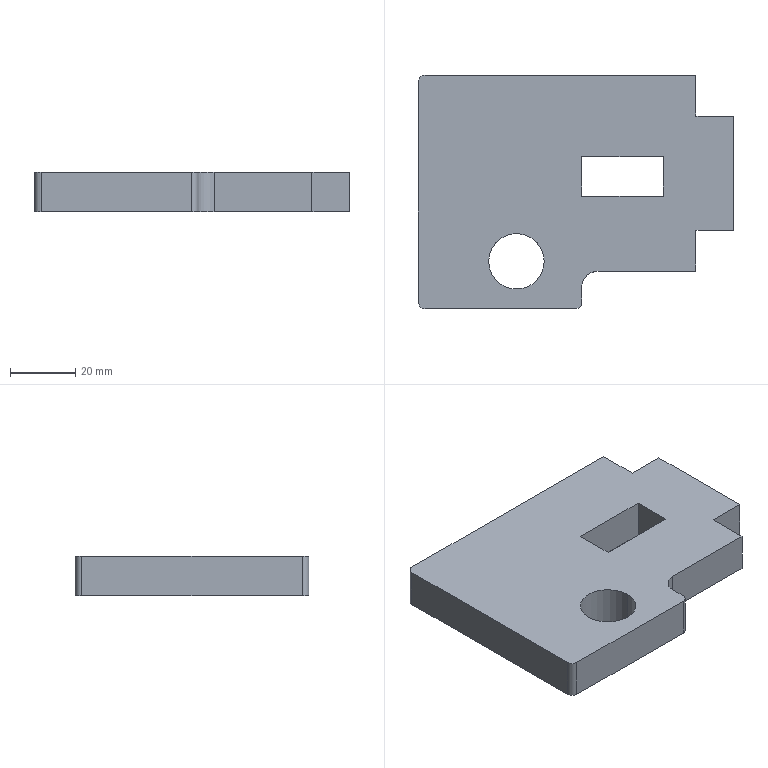Part | SolidWorks | features FlatPattern 1, SMBaseFlange 1, SheetMetal 1 | 1 solid | 22 faces | box 96.5 x 71.502 x 12 mm | volume 66641 mm3 | plane 16 | cylinder 6 | commonest cylinder face diameters 4 x3 17 x2 10 x1
STEP:
#1=CARTESIAN_POINT('',(-26.5,-18.,12.));
#2=VERTEX_POINT('',#1);
#3=CARTESIAN_POINT('',(-9.5,-18.,12.));
#4=VERTEX_POINT('',#3);
#5=CARTESIAN_POINT('',(-18.,-18.,12.));
#6=DIRECTION('',(0.,0.,1.));
#7=DIRECTION('',(1.,0.,0.));
#8=AXIS2_PLACEMENT_3D('',#5,#6,#7);
#9=CIRCLE('',#8,8.5);
#10=EDGE_CURVE('',#2,#4,#9,.T.);
#11=ORIENTED_EDGE('',*,*,#10,.T.);
#12=CARTESIAN_POINT('',(-9.5,-18.,0.));
#13=VERTEX_POINT('',#12);
#14=CARTESIAN_POINT('',(-9.5,-18.,12.));
#15=DIRECTION('',(0.,0.,-1.));
#16=VECTOR('',#15,1000.);
#17=LINE('',#14,#16);
#18=EDGE_CURVE('',#4,#13,#17,.T.);
#19=ORIENTED_EDGE('',*,*,#18,.T.);
#20=CARTESIAN_POINT('',(-26.5,-18.,0.));
#21=VERTEX_POINT('',#20);
#22=CARTESIAN_POINT('',(-18.,-18.,0.));
#23=DIRECTION('',(0.,0.,1.));
#24=DIRECTION('',(1.,0.,0.));
#25=AXIS2_PLACEMENT_3D('',#22,#23,#24);
#26=CIRCLE('',#25,8.5);
#27=EDGE_CURVE('',#21,#13,#26,.T.);
#28=ORIENTED_EDGE('',*,*,#27,.F.);
#29=CARTESIAN_POINT('',(-26.5,-18.,12.));
#30=DIRECTION('',(0.,0.,-1.));
#31=VECTOR('',#30,1000.);
#32=LINE('',#29,#31);
#33=EDGE_CURVE('',#2,#21,#32,.T.);
#34=ORIENTED_EDGE('',*,*,#33,.F.);
#35=EDGE_LOOP('',(#11,#19,#28,#34));
#36=FACE_OUTER_BOUND('',#35,.T.);
#37=CARTESIAN_POINT('',(-18.,-18.,12.));
#38=DIRECTION('',(0.,0.,-1.));
#39=DIRECTION('',(-1.,0.,0.));
#40=AXIS2_PLACEMENT_3D('',#37,#38,#39);
#41=CYLINDRICAL_SURFACE('',#40,8.5);
#42=ADVANCED_FACE('',(#36),#41,.F.);
#43=CARTESIAN_POINT('',(48.5,26.502,12.));
#44=VERTEX_POINT('',#43);
#45=CARTESIAN_POINT('',(37.,26.502,12.));
#46=VERTEX_POINT('',#45);
#47=CARTESIAN_POINT('',(48.5,26.502,12.));
#48=DIRECTION('',(-1.,0.,0.));
#49=VECTOR('',#48,1000.);
#50=LINE('',#47,#49);
#51=EDGE_CURVE('',#44,#46,#50,.T.);
#52=ORIENTED_EDGE('',*,*,#51,.T.);
#53=CARTESIAN_POINT('',(37.,39.002,12.));
#54=VERTEX_POINT('',#53);
#55=CARTESIAN_POINT('',(37.,26.502,12.));
#56=DIRECTION('',(0.,1.,0.));
#57=VECTOR('',#56,1000.);
#58=LINE('',#55,#57);
#59=EDGE_CURVE('',#46,#54,#58,.T.);
#60=ORIENTED_EDGE('',*,*,#59,.T.);
#61=CARTESIAN_POINT('',(-46.,39.002,12.));
#62=VERTEX_POINT('',#61);
#63=CARTESIAN_POINT('',(37.,39.002,12.));
#64=DIRECTION('',(-1.,0.,0.));
#65=VECTOR('',#64,1000.);
#66=LINE('',#63,#65);
#67=EDGE_CURVE('',#54,#62,#66,.T.);
#68=ORIENTED_EDGE('',*,*,#67,.T.);
#69=CARTESIAN_POINT('',(-48.,37.002,12.));
#70=VERTEX_POINT('',#69);
#71=CARTESIAN_POINT('',(-46.,37.002,12.));
#72=DIRECTION('',(0.,0.,1.));
#73=DIRECTION('',(1.,0.,0.));
#74=AXIS2_PLACEMENT_3D('',#71,#72,#73);
#75=CIRCLE('',#74,2.);
#76=EDGE_CURVE('',#62,#70,#75,.T.);
#77=ORIENTED_EDGE('',*,*,#76,.T.);
#78=CARTESIAN_POINT('',(-48.,-30.5,12.));
#79=VERTEX_POINT('',#78);
#80=CARTESIAN_POINT('',(-48.,-30.5,12.));
#81=DIRECTION('',(0.,-1.,0.));
#82=VECTOR('',#81,1000.);
#83=LINE('',#80,#82);
#84=EDGE_CURVE('',#70,#79,#83,.T.);
#85=ORIENTED_EDGE('',*,*,#84,.T.);
#86=CARTESIAN_POINT('',(-46.,-32.5,12.));
#87=VERTEX_POINT('',#86);
#88=CARTESIAN_POINT('',(-46.,-30.5,12.));
#89=DIRECTION('',(0.,0.,1.));
#90=DIRECTION('',(1.,0.,0.));
#91=AXIS2_PLACEMENT_3D('',#88,#89,#90);
#92=CIRCLE('',#91,2.);
#93=EDGE_CURVE('',#79,#87,#92,.T.);
#94=ORIENTED_EDGE('',*,*,#93,.T.);
#95=CARTESIAN_POINT('',(0.,-32.5,12.));
#96=VERTEX_POINT('',#95);
#97=CARTESIAN_POINT('',(-46.,-32.5,12.));
#98=DIRECTION('',(1.,0.,0.));
#99=VECTOR('',#98,1000.);
#100=LINE('',#97,#99);
#101=EDGE_CURVE('',#87,#96,#100,.T.);
#102=ORIENTED_EDGE('',*,*,#101,.T.);
#103=CARTESIAN_POINT('',(2.,-30.5,12.));
#104=VERTEX_POINT('',#103);
#105=CARTESIAN_POINT('',(0.,-30.5,12.));
#106=DIRECTION('',(0.,0.,1.));
#107=DIRECTION('',(1.,0.,0.));
#108=AXIS2_PLACEMENT_3D('',#105,#106,#107);
#109=CIRCLE('',#108,2.);
#110=EDGE_CURVE('',#96,#104,#109,.T.);
#111=ORIENTED_EDGE('',*,*,#110,.T.);
#112=CARTESIAN_POINT('',(2.,-25.998,12.));
#113=VERTEX_POINT('',#112);
#114=CARTESIAN_POINT('',(2.,-30.5,12.));
#115=DIRECTION('',(0.,1.,0.));
#116=VECTOR('',#115,1000.);
#117=LINE('',#114,#116);
#118=EDGE_CURVE('',#104,#113,#117,.T.);
#119=ORIENTED_EDGE('',*,*,#118,.T.);
#120=CARTESIAN_POINT('',(7.,-20.998,12.));
#121=VERTEX_POINT('',#120);
#122=CARTESIAN_POINT('',(7.,-25.998,12.));
#123=DIRECTION('',(0.,0.,-1.));
#124=DIRECTION('',(1.,0.,0.));
#125=AXIS2_PLACEMENT_3D('',#122,#123,#124);
#126=CIRCLE('',#125,5.);
#127=EDGE_CURVE('',#113,#121,#126,.T.);
#128=ORIENTED_EDGE('',*,*,#127,.T.);
#129=CARTESIAN_POINT('',(37.,-20.998,12.));
#130=VERTEX_POINT('',#129);
#131=CARTESIAN_POINT('',(7.,-20.998,12.));
#132=DIRECTION('',(1.,0.,0.));
#133=VECTOR('',#132,1000.);
#134=LINE('',#131,#133);
#135=EDGE_CURVE('',#121,#130,#134,.T.);
#136=ORIENTED_EDGE('',*,*,#135,.T.);
#137=CARTESIAN_POINT('',(37.,-8.498,12.));
#138=VERTEX_POINT('',#137);
#139=CARTESIAN_POINT('',(37.,-20.998,12.));
#140=DIRECTION('',(0.,1.,0.));
#141=VECTOR('',#140,1000.);
#142=LINE('',#139,#141);
#143=EDGE_CURVE('',#130,#138,#142,.T.);
#144=ORIENTED_EDGE('',*,*,#143,.T.);
#145=CARTESIAN_POINT('',(48.5,-8.498,12.));
#146=VERTEX_POINT('',#145);
#147=CARTESIAN_POINT('',(37.,-8.498,12.));
#148=DIRECTION('',(1.,0.,0.));
#149=VECTOR('',#148,1000.);
#150=LINE('',#147,#149);
#151=EDGE_CURVE('',#138,#146,#150,.T.);
#152=ORIENTED_EDGE('',*,*,#151,.T.);
#153=CARTESIAN_POINT('',(48.5,-8.498,12.));
#154=DIRECTION('',(0.,1.,0.));
#155=VECTOR('',#154,1000.);
#156=LINE('',#153,#155);
#157=EDGE_CURVE('',#146,#44,#156,.T.);
#158=ORIENTED_EDGE('',*,*,#157,.T.);
#159=EDGE_LOOP('',(#52,#60,#68,#77,#85,#94,#102,#111,#119,#128,#136,#144,#152,#158));
#160=FACE_OUTER_BOUND('',#159,.T.);
#161=ORIENTED_EDGE('',*,*,#10,.F.);
#162=CARTESIAN_POINT('',(-18.,-18.,12.));
#163=DIRECTION('',(0.,0.,1.));
#164=DIRECTION('',(1.,0.,0.));
#165=AXIS2_PLACEMENT_3D('',#162,#163,#164);
#166=CIRCLE('',#165,8.5);
#167=EDGE_CURVE('',#4,#2,#166,.T.);
#168=ORIENTED_EDGE('',*,*,#167,.F.);
#169=EDGE_LOOP('',(#161,#168));
#170=FACE_BOUND('',#169,.T.);
#171=CARTESIAN_POINT('',(2.,2.002,12.));
#172=VERTEX_POINT('',#171);
#173=CARTESIAN_POINT('',(27.,2.002,12.));
#174=VERTEX_POINT('',#173);
#175=CARTESIAN_POINT('',(2.,2.002,12.));
#176=DIRECTION('',(1.,0.,0.));
#177=VECTOR('',#176,1000.);
#178=LINE('',#175,#177);
#179=EDGE_CURVE('',#172,#174,#178,.T.);
#180=ORIENTED_EDGE('',*,*,#179,.F.);
#181=CARTESIAN_POINT('',(2.,14.002,12.));
#182=VERTEX_POINT('',#181);
#183=CARTESIAN_POINT('',(2.,14.002,12.));
#184=DIRECTION('',(0.,-1.,0.));
#185=VECTOR('',#184,1000.);
#186=LINE('',#183,#185);
#187=EDGE_CURVE('',#182,#172,#186,.T.);
#188=ORIENTED_EDGE('',*,*,#187,.F.);
#189=CARTESIAN_POINT('',(27.,14.002,12.));
#190=VERTEX_POINT('',#189);
#191=CARTESIAN_POINT('',(2.,14.002,12.));
#192=DIRECTION('',(-1.,0.,0.));
#193=VECTOR('',#192,1000.);
#194=LINE('',#191,#193);
#195=EDGE_CURVE('',#190,#182,#194,.T.);
#196=ORIENTED_EDGE('',*,*,#195,.F.);
#197=CARTESIAN_POINT('',(27.,14.002,12.));
#198=DIRECTION('',(0.,1.,0.));
#199=VECTOR('',#198,1000.);
#200=LINE('',#197,#199);
#201=EDGE_CURVE('',#174,#190,#200,.T.);
#202=ORIENTED_EDGE('',*,*,#201,.F.);
#203=EDGE_LOOP('',(#180,#188,#196,#202));
#204=FACE_BOUND('',#203,.T.);
#205=CARTESIAN_POINT('',(-46.,37.002,12.));
#206=DIRECTION('',(0.,0.,1.));
#207=DIRECTION('',(1.,0.,0.));
#208=AXIS2_PLACEMENT_3D('',#205,#206,#207);
#209=PLANE('',#208);
#210=ADVANCED_FACE('',(#160,#170,#204),#209,.T.);
#211=ORIENTED_EDGE('',*,*,#27,.T.);
#212=CARTESIAN_POINT('',(-18.,-18.,0.));
#213=DIRECTION('',(0.,0.,1.));
#214=DIRECTION('',(1.,0.,0.));
#215=AXIS2_PLACEMENT_3D('',#212,#213,#214);
#216=CIRCLE('',#215,8.5);
#217=EDGE_CURVE('',#13,#21,#216,.T.);
#218=ORIENTED_EDGE('',*,*,#217,.T.);
#219=EDGE_LOOP('',(#211,#218));
#220=FACE_BOUND('',#219,.T.);
#221=CARTESIAN_POINT('',(48.5,26.502,0.));
#222=VERTEX_POINT('',#221);
#223=CARTESIAN_POINT('',(37.,26.502,0.));
#224=VERTEX_POINT('',#223);
#225=CARTESIAN_POINT('',(48.5,26.502,0.));
#226=DIRECTION('',(-1.,0.,0.));
#227=VECTOR('',#226,1000.);
#228=LINE('',#225,#227);
#229=EDGE_CURVE('',#222,#224,#228,.T.);
#230=ORIENTED_EDGE('',*,*,#229,.F.);
#231=CARTESIAN_POINT('',(48.5,-8.498,0.));
#232=VERTEX_POINT('',#231);
#233=CARTESIAN_POINT('',(48.5,-8.498,0.));
#234=DIRECTION('',(0.,1.,0.));
#235=VECTOR('',#234,1000.);
#236=LINE('',#233,#235);
#237=EDGE_CURVE('',#232,#222,#236,.T.);
#238=ORIENTED_EDGE('',*,*,#237,.F.);
#239=CARTESIAN_POINT('',(37.,-8.498,0.));
#240=VERTEX_POINT('',#239);
#241=CARTESIAN_POINT('',(37.,-8.498,0.));
#242=DIRECTION('',(1.,0.,0.));
#243=VECTOR('',#242,1000.);
#244=LINE('',#241,#243);
#245=EDGE_CURVE('',#240,#232,#244,.T.);
#246=ORIENTED_EDGE('',*,*,#245,.F.);
#247=CARTESIAN_POINT('',(37.,-20.998,0.));
#248=VERTEX_POINT('',#247);
#249=CARTESIAN_POINT('',(37.,-20.998,0.));
#250=DIRECTION('',(0.,1.,0.));
#251=VECTOR('',#250,1000.);
#252=LINE('',#249,#251);
#253=EDGE_CURVE('',#248,#240,#252,.T.);
#254=ORIENTED_EDGE('',*,*,#253,.F.);
#255=CARTESIAN_POINT('',(7.,-20.998,0.));
#256=VERTEX_POINT('',#255);
#257=CARTESIAN_POINT('',(7.,-20.998,0.));
#258=DIRECTION('',(1.,0.,0.));
#259=VECTOR('',#258,1000.);
#260=LINE('',#257,#259);
#261=EDGE_CURVE('',#256,#248,#260,.T.);
#262=ORIENTED_EDGE('',*,*,#261,.F.);
#263=CARTESIAN_POINT('',(2.,-25.998,0.));
#264=VERTEX_POINT('',#263);
#265=CARTESIAN_POINT('',(7.,-25.998,0.));
#266=DIRECTION('',(0.,0.,-1.));
#267=DIRECTION('',(1.,0.,0.));
#268=AXIS2_PLACEMENT_3D('',#265,#266,#267);
#269=CIRCLE('',#268,5.);
#270=EDGE_CURVE('',#264,#256,#269,.T.);
#271=ORIENTED_EDGE('',*,*,#270,.F.);
#272=CARTESIAN_POINT('',(2.,-30.5,0.));
#273=VERTEX_POINT('',#272);
#274=CARTESIAN_POINT('',(2.,-30.5,0.));
#275=DIRECTION('',(0.,1.,0.));
#276=VECTOR('',#275,1000.);
#277=LINE('',#274,#276);
#278=EDGE_CURVE('',#273,#264,#277,.T.);
#279=ORIENTED_EDGE('',*,*,#278,.F.);
#280=CARTESIAN_POINT('',(0.,-32.5,0.));
#281=VERTEX_POINT('',#280);
#282=CARTESIAN_POINT('',(0.,-30.5,0.));
#283=DIRECTION('',(0.,0.,1.));
#284=DIRECTION('',(1.,0.,0.));
#285=AXIS2_PLACEMENT_3D('',#282,#283,#284);
#286=CIRCLE('',#285,2.);
#287=EDGE_CURVE('',#281,#273,#286,.T.);
#288=ORIENTED_EDGE('',*,*,#287,.F.);
#289=CARTESIAN_POINT('',(-46.,-32.5,0.));
#290=VERTEX_POINT('',#289);
#291=CARTESIAN_POINT('',(-46.,-32.5,0.));
#292=DIRECTION('',(1.,0.,0.));
#293=VECTOR('',#292,1000.);
#294=LINE('',#291,#293);
#295=EDGE_CURVE('',#290,#281,#294,.T.);
#296=ORIENTED_EDGE('',*,*,#295,.F.);
#297=CARTESIAN_POINT('',(-48.,-30.5,0.));
#298=VERTEX_POINT('',#297);
#299=CARTESIAN_POINT('',(-46.,-30.5,0.));
#300=DIRECTION('',(0.,0.,1.));
#301=DIRECTION('',(1.,0.,0.));
#302=AXIS2_PLACEMENT_3D('',#299,#300,#301);
#303=CIRCLE('',#302,2.);
#304=EDGE_CURVE('',#298,#290,#303,.T.);
#305=ORIENTED_EDGE('',*,*,#304,.F.);
#306=CARTESIAN_POINT('',(-48.,37.002,0.));
#307=VERTEX_POINT('',#306);
#308=CARTESIAN_POINT('',(-48.,-30.5,0.));
#309=DIRECTION('',(0.,-1.,0.));
#310=VECTOR('',#309,1000.);
#311=LINE('',#308,#310);
#312=EDGE_CURVE('',#307,#298,#311,.T.);
#313=ORIENTED_EDGE('',*,*,#312,.F.);
#314=CARTESIAN_POINT('',(-46.,39.002,0.));
#315=VERTEX_POINT('',#314);
#316=CARTESIAN_POINT('',(-46.,37.002,0.));
#317=DIRECTION('',(0.,0.,1.));
#318=DIRECTION('',(1.,0.,0.));
#319=AXIS2_PLACEMENT_3D('',#316,#317,#318);
#320=CIRCLE('',#319,2.);
#321=EDGE_CURVE('',#315,#307,#320,.T.);
#322=ORIENTED_EDGE('',*,*,#321,.F.);
#323=CARTESIAN_POINT('',(37.,39.002,0.));
#324=VERTEX_POINT('',#323);
#325=CARTESIAN_POINT('',(37.,39.002,0.));
#326=DIRECTION('',(-1.,0.,0.));
#327=VECTOR('',#326,1000.);
#328=LINE('',#325,#327);
#329=EDGE_CURVE('',#324,#315,#328,.T.);
#330=ORIENTED_EDGE('',*,*,#329,.F.);
#331=CARTESIAN_POINT('',(37.,26.502,0.));
#332=DIRECTION('',(0.,1.,0.));
#333=VECTOR('',#332,1000.);
#334=LINE('',#331,#333);
#335=EDGE_CURVE('',#224,#324,#334,.T.);
#336=ORIENTED_EDGE('',*,*,#335,.F.);
#337=EDGE_LOOP('',(#230,#238,#246,#254,#262,#271,#279,#288,#296,#305,#313,#322,#330,#336));
#338=FACE_OUTER_BOUND('',#337,.T.);
#339=CARTESIAN_POINT('',(2.,14.002,0.));
#340=VERTEX_POINT('',#339);
#341=CARTESIAN_POINT('',(2.,2.002,0.));
#342=VERTEX_POINT('',#341);
#343=CARTESIAN_POINT('',(2.,14.002,0.));
#344=DIRECTION('',(0.,-1.,0.));
#345=VECTOR('',#344,1000.);
#346=LINE('',#343,#345);
#347=EDGE_CURVE('',#340,#342,#346,.T.);
#348=ORIENTED_EDGE('',*,*,#347,.T.);
#349=CARTESIAN_POINT('',(27.,2.002,0.));
#350=VERTEX_POINT('',#349);
#351=CARTESIAN_POINT('',(2.,2.002,0.));
#352=DIRECTION('',(1.,0.,0.));
#353=VECTOR('',#352,1000.);
#354=LINE('',#351,#353);
#355=EDGE_CURVE('',#342,#350,#354,.T.);
#356=ORIENTED_EDGE('',*,*,#355,.T.);
#357=CARTESIAN_POINT('',(27.,14.002,0.));
#358=VERTEX_POINT('',#357);
#359=CARTESIAN_POINT('',(27.,14.002,0.));
#360=DIRECTION('',(0.,1.,0.));
#361=VECTOR('',#360,1000.);
#362=LINE('',#359,#361);
#363=EDGE_CURVE('',#350,#358,#362,.T.);
#364=ORIENTED_EDGE('',*,*,#363,.T.);
#365=CARTESIAN_POINT('',(2.,14.002,0.));
#366=DIRECTION('',(-1.,0.,0.));
#367=VECTOR('',#366,1000.);
#368=LINE('',#365,#367);
#369=EDGE_CURVE('',#358,#340,#368,.T.);
#370=ORIENTED_EDGE('',*,*,#369,.T.);
#371=EDGE_LOOP('',(#348,#356,#364,#370));
#372=FACE_BOUND('',#371,.T.);
#373=CARTESIAN_POINT('',(-46.,37.002,0.));
#374=DIRECTION('',(0.,0.,1.));
#375=DIRECTION('',(1.,0.,0.));
#376=AXIS2_PLACEMENT_3D('',#373,#374,#375);
#377=PLANE('',#376);
#378=ADVANCED_FACE('',(#220,#338,#372),#377,.F.);
#379=ORIENTED_EDGE('',*,*,#229,.T.);
#380=CARTESIAN_POINT('',(37.,26.502,12.));
#381=DIRECTION('',(0.,0.,-1.));
#382=VECTOR('',#381,1000.);
#383=LINE('',#380,#382);
#384=EDGE_CURVE('',#46,#224,#383,.T.);
#385=ORIENTED_EDGE('',*,*,#384,.F.);
#386=ORIENTED_EDGE('',*,*,#51,.F.);
#387=CARTESIAN_POINT('',(48.5,26.502,12.));
#388=DIRECTION('',(0.,0.,-1.));
#389=VECTOR('',#388,1000.);
#390=LINE('',#387,#389);
#391=EDGE_CURVE('',#44,#222,#390,.T.);
#392=ORIENTED_EDGE('',*,*,#391,.T.);
#393=EDGE_LOOP('',(#379,#385,#386,#392));
#394=FACE_OUTER_BOUND('',#393,.T.);
#395=CARTESIAN_POINT('',(48.5,26.502,12.));
#396=DIRECTION('',(0.,-1.,0.));
#397=DIRECTION('',(0.,0.,-1.));
#398=AXIS2_PLACEMENT_3D('',#395,#396,#397);
#399=PLANE('',#398);
#400=ADVANCED_FACE('',(#394),#399,.F.);
#401=ORIENTED_EDGE('',*,*,#335,.T.);
#402=CARTESIAN_POINT('',(37.,39.002,12.));
#403=DIRECTION('',(0.,0.,-1.));
#404=VECTOR('',#403,1000.);
#405=LINE('',#402,#404);
#406=EDGE_CURVE('',#54,#324,#405,.T.);
#407=ORIENTED_EDGE('',*,*,#406,.F.);
#408=ORIENTED_EDGE('',*,*,#59,.F.);
#409=ORIENTED_EDGE('',*,*,#384,.T.);
#410=EDGE_LOOP('',(#401,#407,#408,#409));
#411=FACE_OUTER_BOUND('',#410,.T.);
#412=CARTESIAN_POINT('',(37.,26.502,12.));
#413=DIRECTION('',(-1.,0.,0.));
#414=DIRECTION('',(0.,0.,1.));
#415=AXIS2_PLACEMENT_3D('',#412,#413,#414);
#416=PLANE('',#415);
#417=ADVANCED_FACE('',(#411),#416,.F.);
#418=ORIENTED_EDGE('',*,*,#329,.T.);
#419=CARTESIAN_POINT('',(-46.,39.002,12.));
#420=DIRECTION('',(0.,0.,-1.));
#421=VECTOR('',#420,1000.);
#422=LINE('',#419,#421);
#423=EDGE_CURVE('',#62,#315,#422,.T.);
#424=ORIENTED_EDGE('',*,*,#423,.F.);
#425=ORIENTED_EDGE('',*,*,#67,.F.);
#426=ORIENTED_EDGE('',*,*,#406,.T.);
#427=EDGE_LOOP('',(#418,#424,#425,#426));
#428=FACE_OUTER_BOUND('',#427,.T.);
#429=CARTESIAN_POINT('',(37.,39.002,12.));
#430=DIRECTION('',(0.,-1.,0.));
#431=DIRECTION('',(0.,0.,-1.));
#432=AXIS2_PLACEMENT_3D('',#429,#430,#431);
#433=PLANE('',#432);
#434=ADVANCED_FACE('',(#428),#433,.F.);
#435=ORIENTED_EDGE('',*,*,#321,.T.);
#436=CARTESIAN_POINT('',(-48.,37.002,12.));
#437=DIRECTION('',(0.,0.,-1.));
#438=VECTOR('',#437,1000.);
#439=LINE('',#436,#438);
#440=EDGE_CURVE('',#70,#307,#439,.T.);
#441=ORIENTED_EDGE('',*,*,#440,.F.);
#442=ORIENTED_EDGE('',*,*,#76,.F.);
#443=ORIENTED_EDGE('',*,*,#423,.T.);
#444=EDGE_LOOP('',(#435,#441,#442,#443));
#445=FACE_OUTER_BOUND('',#444,.T.);
#446=CARTESIAN_POINT('',(-46.,37.002,12.));
#447=DIRECTION('',(0.,0.,-1.));
#448=DIRECTION('',(-1.,0.,0.));
#449=AXIS2_PLACEMENT_3D('',#446,#447,#448);
#450=CYLINDRICAL_SURFACE('',#449,2.);
#451=ADVANCED_FACE('',(#445),#450,.T.);
#452=ORIENTED_EDGE('',*,*,#312,.T.);
#453=CARTESIAN_POINT('',(-48.,-30.5,12.));
#454=DIRECTION('',(0.,0.,-1.));
#455=VECTOR('',#454,1000.);
#456=LINE('',#453,#455);
#457=EDGE_CURVE('',#79,#298,#456,.T.);
#458=ORIENTED_EDGE('',*,*,#457,.F.);
#459=ORIENTED_EDGE('',*,*,#84,.F.);
#460=ORIENTED_EDGE('',*,*,#440,.T.);
#461=EDGE_LOOP('',(#452,#458,#459,#460));
#462=FACE_OUTER_BOUND('',#461,.T.);
#463=CARTESIAN_POINT('',(-48.,-30.5,12.));
#464=DIRECTION('',(1.,0.,0.));
#465=DIRECTION('',(0.,0.,-1.));
#466=AXIS2_PLACEMENT_3D('',#463,#464,#465);
#467=PLANE('',#466);
#468=ADVANCED_FACE('',(#462),#467,.F.);
#469=ORIENTED_EDGE('',*,*,#304,.T.);
#470=CARTESIAN_POINT('',(-46.,-32.5,12.));
#471=DIRECTION('',(0.,0.,-1.));
#472=VECTOR('',#471,1000.);
#473=LINE('',#470,#472);
#474=EDGE_CURVE('',#87,#290,#473,.T.);
#475=ORIENTED_EDGE('',*,*,#474,.F.);
#476=ORIENTED_EDGE('',*,*,#93,.F.);
#477=ORIENTED_EDGE('',*,*,#457,.T.);
#478=EDGE_LOOP('',(#469,#475,#476,#477));
#479=FACE_OUTER_BOUND('',#478,.T.);
#480=CARTESIAN_POINT('',(-46.,-30.5,12.));
#481=DIRECTION('',(0.,0.,-1.));
#482=DIRECTION('',(-1.,0.,0.));
#483=AXIS2_PLACEMENT_3D('',#480,#481,#482);
#484=CYLINDRICAL_SURFACE('',#483,2.);
#485=ADVANCED_FACE('',(#479),#484,.T.);
#486=ORIENTED_EDGE('',*,*,#295,.T.);
#487=CARTESIAN_POINT('',(0.,-32.5,12.));
#488=DIRECTION('',(0.,0.,-1.));
#489=VECTOR('',#488,1000.);
#490=LINE('',#487,#489);
#491=EDGE_CURVE('',#96,#281,#490,.T.);
#492=ORIENTED_EDGE('',*,*,#491,.F.);
#493=ORIENTED_EDGE('',*,*,#101,.F.);
#494=ORIENTED_EDGE('',*,*,#474,.T.);
#495=EDGE_LOOP('',(#486,#492,#493,#494));
#496=FACE_OUTER_BOUND('',#495,.T.);
#497=CARTESIAN_POINT('',(-46.,-32.5,12.));
#498=DIRECTION('',(0.,1.,0.));
#499=DIRECTION('',(-1.,0.,0.));
#500=AXIS2_PLACEMENT_3D('',#497,#498,#499);
#501=PLANE('',#500);
#502=ADVANCED_FACE('',(#496),#501,.F.);
#503=ORIENTED_EDGE('',*,*,#287,.T.);
#504=CARTESIAN_POINT('',(2.,-30.5,12.));
#505=DIRECTION('',(0.,0.,-1.));
#506=VECTOR('',#505,1000.);
#507=LINE('',#504,#506);
#508=EDGE_CURVE('',#104,#273,#507,.T.);
#509=ORIENTED_EDGE('',*,*,#508,.F.);
#510=ORIENTED_EDGE('',*,*,#110,.F.);
#511=ORIENTED_EDGE('',*,*,#491,.T.);
#512=EDGE_LOOP('',(#503,#509,#510,#511));
#513=FACE_OUTER_BOUND('',#512,.T.);
#514=CARTESIAN_POINT('',(0.,-30.5,12.));
#515=DIRECTION('',(0.,0.,-1.));
#516=DIRECTION('',(-1.,0.,0.));
#517=AXIS2_PLACEMENT_3D('',#514,#515,#516);
#518=CYLINDRICAL_SURFACE('',#517,2.);
#519=ADVANCED_FACE('',(#513),#518,.T.);
#520=ORIENTED_EDGE('',*,*,#278,.T.);
#521=CARTESIAN_POINT('',(2.,-25.998,12.));
#522=DIRECTION('',(0.,0.,-1.));
#523=VECTOR('',#522,1000.);
#524=LINE('',#521,#523);
#525=EDGE_CURVE('',#113,#264,#524,.T.);
#526=ORIENTED_EDGE('',*,*,#525,.F.);
#527=ORIENTED_EDGE('',*,*,#118,.F.);
#528=ORIENTED_EDGE('',*,*,#508,.T.);
#529=EDGE_LOOP('',(#520,#526,#527,#528));
#530=FACE_OUTER_BOUND('',#529,.T.);
#531=CARTESIAN_POINT('',(2.,-30.5,12.));
#532=DIRECTION('',(-1.,0.,0.));
#533=DIRECTION('',(0.,-1.,0.));
#534=AXIS2_PLACEMENT_3D('',#531,#532,#533);
#535=PLANE('',#534);
#536=ADVANCED_FACE('',(#530),#535,.F.);
#537=ORIENTED_EDGE('',*,*,#270,.T.);
#538=CARTESIAN_POINT('',(7.,-20.998,12.));
#539=DIRECTION('',(0.,0.,-1.));
#540=VECTOR('',#539,1000.);
#541=LINE('',#538,#540);
#542=EDGE_CURVE('',#121,#256,#541,.T.);
#543=ORIENTED_EDGE('',*,*,#542,.F.);
#544=ORIENTED_EDGE('',*,*,#127,.F.);
#545=ORIENTED_EDGE('',*,*,#525,.T.);
#546=EDGE_LOOP('',(#537,#543,#544,#545));
#547=FACE_OUTER_BOUND('',#546,.T.);
#548=CARTESIAN_POINT('',(7.,-25.998,12.));
#549=DIRECTION('',(0.,0.,-1.));
#550=DIRECTION('',(-1.,0.,0.));
#551=AXIS2_PLACEMENT_3D('',#548,#549,#550);
#552=CYLINDRICAL_SURFACE('',#551,5.);
#553=ADVANCED_FACE('',(#547),#552,.F.);
#554=ORIENTED_EDGE('',*,*,#261,.T.);
#555=CARTESIAN_POINT('',(37.,-20.998,12.));
#556=DIRECTION('',(0.,0.,-1.));
#557=VECTOR('',#556,1000.);
#558=LINE('',#555,#557);
#559=EDGE_CURVE('',#130,#248,#558,.T.);
#560=ORIENTED_EDGE('',*,*,#559,.F.);
#561=ORIENTED_EDGE('',*,*,#135,.F.);
#562=ORIENTED_EDGE('',*,*,#542,.T.);
#563=EDGE_LOOP('',(#554,#560,#561,#562));
#564=FACE_OUTER_BOUND('',#563,.T.);
#565=CARTESIAN_POINT('',(7.,-20.998,12.));
#566=DIRECTION('',(0.,1.,0.));
#567=DIRECTION('',(-1.,0.,0.));
#568=AXIS2_PLACEMENT_3D('',#565,#566,#567);
#569=PLANE('',#568);
#570=ADVANCED_FACE('',(#564),#569,.F.);
#571=ORIENTED_EDGE('',*,*,#253,.T.);
#572=CARTESIAN_POINT('',(37.,-8.498,12.));
#573=DIRECTION('',(0.,0.,-1.));
#574=VECTOR('',#573,1000.);
#575=LINE('',#572,#574);
#576=EDGE_CURVE('',#138,#240,#575,.T.);
#577=ORIENTED_EDGE('',*,*,#576,.F.);
#578=ORIENTED_EDGE('',*,*,#143,.F.);
#579=ORIENTED_EDGE('',*,*,#559,.T.);
#580=EDGE_LOOP('',(#571,#577,#578,#579));
#581=FACE_OUTER_BOUND('',#580,.T.);
#582=CARTESIAN_POINT('',(37.,-20.998,12.));
#583=DIRECTION('',(-1.,0.,0.));
#584=DIRECTION('',(0.,0.,1.));
#585=AXIS2_PLACEMENT_3D('',#582,#583,#584);
#586=PLANE('',#585);
#587=ADVANCED_FACE('',(#581),#586,.F.);
#588=ORIENTED_EDGE('',*,*,#245,.T.);
#589=CARTESIAN_POINT('',(48.5,-8.498,12.));
#590=DIRECTION('',(0.,0.,-1.));
#591=VECTOR('',#590,1000.);
#592=LINE('',#589,#591);
#593=EDGE_CURVE('',#146,#232,#592,.T.);
#594=ORIENTED_EDGE('',*,*,#593,.F.);
#595=ORIENTED_EDGE('',*,*,#151,.F.);
#596=ORIENTED_EDGE('',*,*,#576,.T.);
#597=EDGE_LOOP('',(#588,#594,#595,#596));
#598=FACE_OUTER_BOUND('',#597,.T.);
#599=CARTESIAN_POINT('',(37.,-8.498,12.));
#600=DIRECTION('',(0.,1.,0.));
#601=DIRECTION('',(0.,0.,1.));
#602=AXIS2_PLACEMENT_3D('',#599,#600,#601);
#603=PLANE('',#602);
#604=ADVANCED_FACE('',(#598),#603,.F.);
#605=ORIENTED_EDGE('',*,*,#237,.T.);
#606=ORIENTED_EDGE('',*,*,#391,.F.);
#607=ORIENTED_EDGE('',*,*,#157,.F.);
#608=ORIENTED_EDGE('',*,*,#593,.T.);
#609=EDGE_LOOP('',(#605,#606,#607,#608));
#610=FACE_OUTER_BOUND('',#609,.T.);
#611=CARTESIAN_POINT('',(48.5,-8.498,12.));
#612=DIRECTION('',(-1.,0.,0.));
#613=DIRECTION('',(0.,0.,1.));
#614=AXIS2_PLACEMENT_3D('',#611,#612,#613);
#615=PLANE('',#614);
#616=ADVANCED_FACE('',(#610),#615,.F.);
#617=ORIENTED_EDGE('',*,*,#18,.F.);
#618=ORIENTED_EDGE('',*,*,#167,.T.);
#619=ORIENTED_EDGE('',*,*,#33,.T.);
#620=ORIENTED_EDGE('',*,*,#217,.F.);
#621=EDGE_LOOP('',(#617,#618,#619,#620));
#622=FACE_OUTER_BOUND('',#621,.T.);
#623=CARTESIAN_POINT('',(-18.,-18.,12.));
#624=DIRECTION('',(0.,0.,-1.));
#625=DIRECTION('',(-1.,0.,0.));
#626=AXIS2_PLACEMENT_3D('',#623,#624,#625);
#627=CYLINDRICAL_SURFACE('',#626,8.5);
#628=ADVANCED_FACE('',(#622),#627,.F.);
#629=ORIENTED_EDGE('',*,*,#347,.F.);
#630=CARTESIAN_POINT('',(2.,14.002,12.));
#631=DIRECTION('',(0.,0.,-1.));
#632=VECTOR('',#631,1000.);
#633=LINE('',#630,#632);
#634=EDGE_CURVE('',#182,#340,#633,.T.);
#635=ORIENTED_EDGE('',*,*,#634,.F.);
#636=ORIENTED_EDGE('',*,*,#187,.T.);
#637=CARTESIAN_POINT('',(2.,2.002,12.));
#638=DIRECTION('',(0.,0.,-1.));
#639=VECTOR('',#638,1000.);
#640=LINE('',#637,#639);
#641=EDGE_CURVE('',#172,#342,#640,.T.);
#642=ORIENTED_EDGE('',*,*,#641,.T.);
#643=EDGE_LOOP('',(#629,#635,#636,#642));
#644=FACE_OUTER_BOUND('',#643,.T.);
#645=CARTESIAN_POINT('',(2.,14.002,12.));
#646=DIRECTION('',(1.,0.,0.));
#647=DIRECTION('',(0.,0.,-1.));
#648=AXIS2_PLACEMENT_3D('',#645,#646,#647);
#649=PLANE('',#648);
#650=ADVANCED_FACE('',(#644),#649,.T.);
#651=ORIENTED_EDGE('',*,*,#355,.F.);
#652=ORIENTED_EDGE('',*,*,#641,.F.);
#653=ORIENTED_EDGE('',*,*,#179,.T.);
#654=CARTESIAN_POINT('',(27.,2.002,12.));
#655=DIRECTION('',(0.,0.,-1.));
#656=VECTOR('',#655,1000.);
#657=LINE('',#654,#656);
#658=EDGE_CURVE('',#174,#350,#657,.T.);
#659=ORIENTED_EDGE('',*,*,#658,.T.);
#660=EDGE_LOOP('',(#651,#652,#653,#659));
#661=FACE_OUTER_BOUND('',#660,.T.);
#662=CARTESIAN_POINT('',(2.,2.002,12.));
#663=DIRECTION('',(0.,1.,0.));
#664=DIRECTION('',(0.,0.,1.));
#665=AXIS2_PLACEMENT_3D('',#662,#663,#664);
#666=PLANE('',#665);
#667=ADVANCED_FACE('',(#661),#666,.T.);
#668=ORIENTED_EDGE('',*,*,#363,.F.);
#669=ORIENTED_EDGE('',*,*,#658,.F.);
#670=ORIENTED_EDGE('',*,*,#201,.T.);
#671=CARTESIAN_POINT('',(27.,14.002,12.));
#672=DIRECTION('',(0.,0.,-1.));
#673=VECTOR('',#672,1000.);
#674=LINE('',#671,#673);
#675=EDGE_CURVE('',#190,#358,#674,.T.);
#676=ORIENTED_EDGE('',*,*,#675,.T.);
#677=EDGE_LOOP('',(#668,#669,#670,#676));
#678=FACE_OUTER_BOUND('',#677,.T.);
#679=CARTESIAN_POINT('',(27.,14.002,12.));
#680=DIRECTION('',(-1.,0.,0.));
#681=DIRECTION('',(0.,0.,1.));
#682=AXIS2_PLACEMENT_3D('',#679,#680,#681);
#683=PLANE('',#682);
#684=ADVANCED_FACE('',(#678),#683,.T.);
#685=ORIENTED_EDGE('',*,*,#369,.F.);
#686=ORIENTED_EDGE('',*,*,#675,.F.);
#687=ORIENTED_EDGE('',*,*,#195,.T.);
#688=ORIENTED_EDGE('',*,*,#634,.T.);
#689=EDGE_LOOP('',(#685,#686,#687,#688));
#690=FACE_OUTER_BOUND('',#689,.T.);
#691=CARTESIAN_POINT('',(2.,14.002,12.));
#692=DIRECTION('',(0.,-1.,0.));
#693=DIRECTION('',(0.,0.,-1.));
#694=AXIS2_PLACEMENT_3D('',#691,#692,#693);
#695=PLANE('',#694);
#696=ADVANCED_FACE('',(#690),#695,.T.);
#697=CLOSED_SHELL('',(#42,#210,#378,#400,#417,#434,#451,#468,#485,#502,#519,#536,#553,#570,#587,#604,#616,#628,#650,#667,#684,#696));
#698=MANIFOLD_SOLID_BREP('',#697);
#699=CARTESIAN_POINT('',(0.,0.,0.));
#700=DIRECTION('',(0.,0.,1.));
#701=DIRECTION('',(1.,0.,0.));
#702=AXIS2_PLACEMENT_3D('',#699,#700,#701);
#703=(LENGTH_UNIT()NAMED_UNIT(*)SI_UNIT(.MILLI.,.METRE.));
#704=UNCERTAINTY_MEASURE_WITH_UNIT(LENGTH_MEASURE(0.00001),#703,'','');
#705=(NAMED_UNIT(*)PLANE_ANGLE_UNIT()SI_UNIT($,.RADIAN.));
#706=(NAMED_UNIT(*)SI_UNIT($,.STERADIAN.)SOLID_ANGLE_UNIT());
#707=(GEOMETRIC_REPRESENTATION_CONTEXT(3)GLOBAL_UNCERTAINTY_ASSIGNED_CONTEXT((#704))GLOBAL_UNIT_ASSIGNED_CONTEXT((#703,#705,#706))REPRESENTATION_CONTEXT('',''));
#708=ADVANCED_BREP_SHAPE_REPRESENTATION('',(#698,#702),#707);